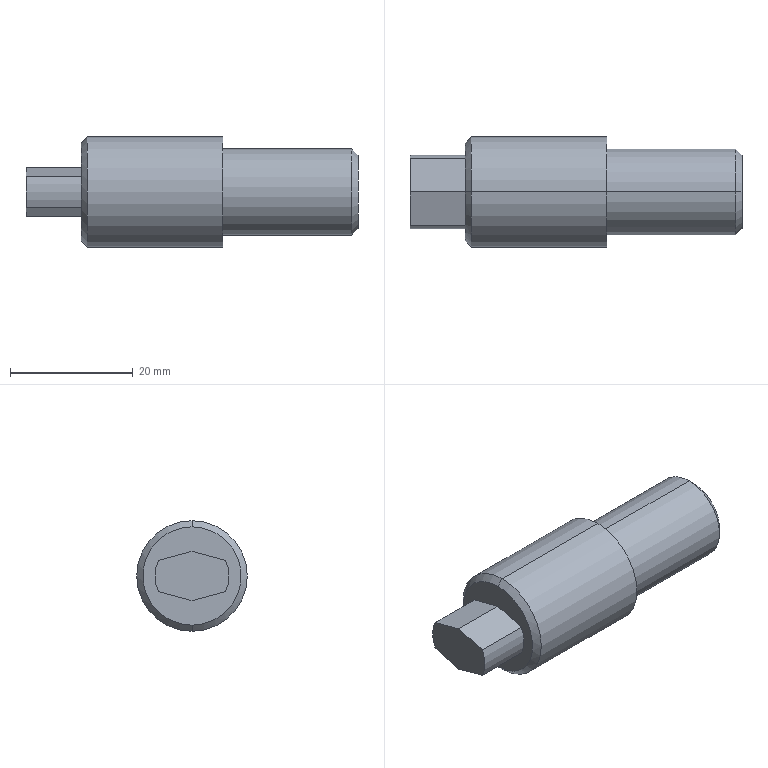Part | SolidWorks | features Chamfer 2, ICE 1, Revolution 1 | 1 solid | 18 faces | box 54 x 18 x 18 mm | volume 9866 mm3 | plane 8 | cylinder 6 | cone 4 | commonest cylinder face diameters 12 x2 14 x2 18 x2
STEP:
#1=CARTESIAN_POINT('',(-21.473,0.,8.));
#2=VERTEX_POINT('',#1);
#3=CARTESIAN_POINT('',(-21.473,0.,-8.));
#4=VERTEX_POINT('',#3);
#5=CARTESIAN_POINT('',(-21.473,0.,0.));
#6=DIRECTION('',(-1.,0.,0.));
#7=DIRECTION('',(0.,0.,-1.));
#8=AXIS2_PLACEMENT_3D('',#5,#6,#7);
#9=CIRCLE('',#8,8.);
#10=EDGE_CURVE('',#2,#4,#9,.T.);
#11=ORIENTED_EDGE('',*,*,#10,.F.);
#12=CARTESIAN_POINT('',(-20.473,0.,9.));
#13=VERTEX_POINT('',#12);
#14=CARTESIAN_POINT('',(-21.473,0.,8.));
#15=DIRECTION('',(0.7071,0.,0.7071));
#16=VECTOR('',#15,1000.);
#17=LINE('',#14,#16);
#18=EDGE_CURVE('',#2,#13,#17,.T.);
#19=ORIENTED_EDGE('',*,*,#18,.T.);
#20=CARTESIAN_POINT('',(-20.473,0.,-9.));
#21=VERTEX_POINT('',#20);
#22=CARTESIAN_POINT('',(-20.473,0.,0.));
#23=DIRECTION('',(1.,0.,0.));
#24=DIRECTION('',(0.,0.,-1.));
#25=AXIS2_PLACEMENT_3D('',#22,#23,#24);
#26=CIRCLE('',#25,9.);
#27=EDGE_CURVE('',#21,#13,#26,.T.);
#28=ORIENTED_EDGE('',*,*,#27,.F.);
#29=CARTESIAN_POINT('',(-21.473,0.,-8.));
#30=DIRECTION('',(0.7071,0.,-0.7071));
#31=VECTOR('',#30,1000.);
#32=LINE('',#29,#31);
#33=EDGE_CURVE('',#4,#21,#32,.T.);
#34=ORIENTED_EDGE('',*,*,#33,.F.);
#35=EDGE_LOOP('',(#11,#19,#28,#34));
#36=FACE_OUTER_BOUND('',#35,.T.);
#37=CARTESIAN_POINT('',(-21.473,0.,0.));
#38=DIRECTION('',(1.,0.,0.));
#39=DIRECTION('',(0.,0.,-1.));
#40=AXIS2_PLACEMENT_3D('',#37,#38,#39);
#41=CONICAL_SURFACE('',#40,8.,0.7854);
#42=ADVANCED_FACE('',(#36),#41,.T.);
#43=CARTESIAN_POINT('',(23.527,0.,-6.));
#44=VERTEX_POINT('',#43);
#45=CARTESIAN_POINT('',(23.527,0.,6.));
#46=VERTEX_POINT('',#45);
#47=CARTESIAN_POINT('',(23.527,0.,0.));
#48=DIRECTION('',(1.,0.,0.));
#49=DIRECTION('',(0.,0.,1.));
#50=AXIS2_PLACEMENT_3D('',#47,#48,#49);
#51=CIRCLE('',#50,6.);
#52=EDGE_CURVE('',#44,#46,#51,.T.);
#53=ORIENTED_EDGE('',*,*,#52,.F.);
#54=CARTESIAN_POINT('',(22.527,0.,-7.));
#55=VERTEX_POINT('',#54);
#56=CARTESIAN_POINT('',(22.527,0.,-7.));
#57=DIRECTION('',(-0.7071,0.,-0.7071));
#58=VECTOR('',#57,1000.);
#59=LINE('',#56,#58);
#60=EDGE_CURVE('',#44,#55,#59,.T.);
#61=ORIENTED_EDGE('',*,*,#60,.T.);
#62=CARTESIAN_POINT('',(22.527,0.,7.));
#63=VERTEX_POINT('',#62);
#64=CARTESIAN_POINT('',(22.527,0.,0.));
#65=DIRECTION('',(-1.,0.,0.));
#66=DIRECTION('',(0.,0.,1.));
#67=AXIS2_PLACEMENT_3D('',#64,#65,#66);
#68=CIRCLE('',#67,7.);
#69=EDGE_CURVE('',#63,#55,#68,.T.);
#70=ORIENTED_EDGE('',*,*,#69,.F.);
#71=CARTESIAN_POINT('',(22.527,0.,7.));
#72=DIRECTION('',(-0.7071,0.,0.7071));
#73=VECTOR('',#72,1000.);
#74=LINE('',#71,#73);
#75=EDGE_CURVE('',#46,#63,#74,.T.);
#76=ORIENTED_EDGE('',*,*,#75,.F.);
#77=EDGE_LOOP('',(#53,#61,#70,#76));
#78=FACE_OUTER_BOUND('',#77,.T.);
#79=CARTESIAN_POINT('',(22.527,0.,0.));
#80=DIRECTION('',(-1.,0.,0.));
#81=DIRECTION('',(0.,0.,1.));
#82=AXIS2_PLACEMENT_3D('',#79,#80,#81);
#83=CONICAL_SURFACE('',#82,7.,0.7854);
#84=ADVANCED_FACE('',(#78),#83,.T.);
#85=ORIENTED_EDGE('',*,*,#69,.T.);
#86=CARTESIAN_POINT('',(1.527,0.,-7.));
#87=VERTEX_POINT('',#86);
#88=CARTESIAN_POINT('',(-65.319,0.,-7.));
#89=DIRECTION('',(-1.,0.,0.));
#90=VECTOR('',#89,1000.);
#91=LINE('',#88,#90);
#92=EDGE_CURVE('',#55,#87,#91,.T.);
#93=ORIENTED_EDGE('',*,*,#92,.T.);
#94=CARTESIAN_POINT('',(1.527,0.,7.));
#95=VERTEX_POINT('',#94);
#96=CARTESIAN_POINT('',(1.527,0.,0.));
#97=DIRECTION('',(-1.,0.,0.));
#98=DIRECTION('',(0.,0.,1.));
#99=AXIS2_PLACEMENT_3D('',#96,#97,#98);
#100=CIRCLE('',#99,7.);
#101=EDGE_CURVE('',#95,#87,#100,.T.);
#102=ORIENTED_EDGE('',*,*,#101,.F.);
#103=CARTESIAN_POINT('',(-65.319,0.,7.));
#104=DIRECTION('',(-1.,0.,0.));
#105=VECTOR('',#104,1000.);
#106=LINE('',#103,#105);
#107=EDGE_CURVE('',#63,#95,#106,.T.);
#108=ORIENTED_EDGE('',*,*,#107,.F.);
#109=EDGE_LOOP('',(#85,#93,#102,#108));
#110=FACE_OUTER_BOUND('',#109,.T.);
#111=CARTESIAN_POINT('',(-65.319,0.,0.));
#112=DIRECTION('',(-1.,0.,0.));
#113=DIRECTION('',(0.,0.,1.));
#114=AXIS2_PLACEMENT_3D('',#111,#112,#113);
#115=CYLINDRICAL_SURFACE('',#114,7.);
#116=ADVANCED_FACE('',(#110),#115,.T.);
#117=CARTESIAN_POINT('',(1.527,0.,9.));
#118=VERTEX_POINT('',#117);
#119=CARTESIAN_POINT('',(1.527,0.,-9.));
#120=VERTEX_POINT('',#119);
#121=CARTESIAN_POINT('',(1.527,0.,0.));
#122=DIRECTION('',(-1.,0.,0.));
#123=DIRECTION('',(0.,0.,1.));
#124=AXIS2_PLACEMENT_3D('',#121,#122,#123);
#125=CIRCLE('',#124,9.);
#126=EDGE_CURVE('',#118,#120,#125,.T.);
#127=ORIENTED_EDGE('',*,*,#126,.T.);
#128=CARTESIAN_POINT('',(-65.319,0.,-9.));
#129=DIRECTION('',(-1.,0.,0.));
#130=VECTOR('',#129,1000.);
#131=LINE('',#128,#130);
#132=EDGE_CURVE('',#120,#21,#131,.T.);
#133=ORIENTED_EDGE('',*,*,#132,.T.);
#134=ORIENTED_EDGE('',*,*,#27,.T.);
#135=CARTESIAN_POINT('',(-65.319,0.,9.));
#136=DIRECTION('',(-1.,0.,0.));
#137=VECTOR('',#136,1000.);
#138=LINE('',#135,#137);
#139=EDGE_CURVE('',#118,#13,#138,.T.);
#140=ORIENTED_EDGE('',*,*,#139,.F.);
#141=EDGE_LOOP('',(#127,#133,#134,#140));
#142=FACE_OUTER_BOUND('',#141,.T.);
#143=CARTESIAN_POINT('',(-65.319,0.,0.));
#144=DIRECTION('',(-1.,0.,0.));
#145=DIRECTION('',(0.,0.,1.));
#146=AXIS2_PLACEMENT_3D('',#143,#144,#145);
#147=CYLINDRICAL_SURFACE('',#146,9.);
#148=ADVANCED_FACE('',(#142),#147,.T.);
#149=CARTESIAN_POINT('',(-21.473,0.,0.));
#150=DIRECTION('',(-1.,0.,0.));
#151=DIRECTION('',(0.,0.,-1.));
#152=AXIS2_PLACEMENT_3D('',#149,#150,#151);
#153=CIRCLE('',#152,8.);
#154=EDGE_CURVE('',#4,#2,#153,.T.);
#155=ORIENTED_EDGE('',*,*,#154,.T.);
#156=ORIENTED_EDGE('',*,*,#10,.T.);
#157=EDGE_LOOP('',(#155,#156));
#158=FACE_OUTER_BOUND('',#157,.T.);
#159=CARTESIAN_POINT('',(-21.473,-5.434,-2.544));
#160=VERTEX_POINT('',#159);
#161=CARTESIAN_POINT('',(-21.473,-5.434,2.544));
#162=VERTEX_POINT('',#161);
#163=CARTESIAN_POINT('',(-21.473,0.,0.));
#164=DIRECTION('',(-1.,0.,0.));
#165=DIRECTION('',(0.,0.,1.));
#166=AXIS2_PLACEMENT_3D('',#163,#164,#165);
#167=CIRCLE('',#166,6.);
#168=EDGE_CURVE('',#160,#162,#167,.T.);
#169=ORIENTED_EDGE('',*,*,#168,.F.);
#170=CARTESIAN_POINT('',(-21.473,0.,-4.));
#171=VERTEX_POINT('',#170);
#172=CARTESIAN_POINT('',(-21.473,0.,-4.));
#173=DIRECTION('',(0.,-0.9659,0.2588));
#174=VECTOR('',#173,1000.);
#175=LINE('',#172,#174);
#176=EDGE_CURVE('',#171,#160,#175,.T.);
#177=ORIENTED_EDGE('',*,*,#176,.F.);
#178=CARTESIAN_POINT('',(-21.473,5.434,-2.544));
#179=VERTEX_POINT('',#178);
#180=CARTESIAN_POINT('',(-21.473,0.,-4.));
#181=DIRECTION('',(0.,-0.9659,-0.2588));
#182=VECTOR('',#181,1000.);
#183=LINE('',#180,#182);
#184=EDGE_CURVE('',#179,#171,#183,.T.);
#185=ORIENTED_EDGE('',*,*,#184,.F.);
#186=CARTESIAN_POINT('',(-21.473,5.434,2.544));
#187=VERTEX_POINT('',#186);
#188=CARTESIAN_POINT('',(-21.473,0.,0.));
#189=DIRECTION('',(-1.,0.,0.));
#190=DIRECTION('',(0.,0.,1.));
#191=AXIS2_PLACEMENT_3D('',#188,#189,#190);
#192=CIRCLE('',#191,6.);
#193=EDGE_CURVE('',#187,#179,#192,.T.);
#194=ORIENTED_EDGE('',*,*,#193,.F.);
#195=CARTESIAN_POINT('',(-21.473,0.,4.));
#196=VERTEX_POINT('',#195);
#197=CARTESIAN_POINT('',(-21.473,0.,4.));
#198=DIRECTION('',(0.,0.9659,-0.2588));
#199=VECTOR('',#198,1000.);
#200=LINE('',#197,#199);
#201=EDGE_CURVE('',#196,#187,#200,.T.);
#202=ORIENTED_EDGE('',*,*,#201,.F.);
#203=CARTESIAN_POINT('',(-21.473,0.,4.));
#204=DIRECTION('',(0.,0.9659,0.2588));
#205=VECTOR('',#204,1000.);
#206=LINE('',#203,#205);
#207=EDGE_CURVE('',#162,#196,#206,.T.);
#208=ORIENTED_EDGE('',*,*,#207,.F.);
#209=EDGE_LOOP('',(#169,#177,#185,#194,#202,#208));
#210=FACE_BOUND('',#209,.T.);
#211=CARTESIAN_POINT('',(-21.473,0.,0.));
#212=DIRECTION('',(1.,0.,0.));
#213=DIRECTION('',(0.,0.,-1.));
#214=AXIS2_PLACEMENT_3D('',#211,#212,#213);
#215=PLANE('',#214);
#216=ADVANCED_FACE('',(#158,#210),#215,.F.);
#217=ORIENTED_EDGE('',*,*,#132,.F.);
#218=CARTESIAN_POINT('',(1.527,0.,0.));
#219=DIRECTION('',(-1.,0.,0.));
#220=DIRECTION('',(0.,0.,1.));
#221=AXIS2_PLACEMENT_3D('',#218,#219,#220);
#222=CIRCLE('',#221,9.);
#223=EDGE_CURVE('',#120,#118,#222,.T.);
#224=ORIENTED_EDGE('',*,*,#223,.T.);
#225=ORIENTED_EDGE('',*,*,#139,.T.);
#226=CARTESIAN_POINT('',(-20.473,0.,0.));
#227=DIRECTION('',(1.,0.,0.));
#228=DIRECTION('',(0.,0.,-1.));
#229=AXIS2_PLACEMENT_3D('',#226,#227,#228);
#230=CIRCLE('',#229,9.);
#231=EDGE_CURVE('',#13,#21,#230,.T.);
#232=ORIENTED_EDGE('',*,*,#231,.T.);
#233=EDGE_LOOP('',(#217,#224,#225,#232));
#234=FACE_OUTER_BOUND('',#233,.T.);
#235=CARTESIAN_POINT('',(-65.319,0.,0.));
#236=DIRECTION('',(-1.,0.,0.));
#237=DIRECTION('',(0.,0.,1.));
#238=AXIS2_PLACEMENT_3D('',#235,#236,#237);
#239=CYLINDRICAL_SURFACE('',#238,9.);
#240=ADVANCED_FACE('',(#234),#239,.T.);
#241=ORIENTED_EDGE('',*,*,#126,.F.);
#242=ORIENTED_EDGE('',*,*,#223,.F.);
#243=EDGE_LOOP('',(#241,#242));
#244=FACE_OUTER_BOUND('',#243,.T.);
#245=ORIENTED_EDGE('',*,*,#101,.T.);
#246=CARTESIAN_POINT('',(1.527,0.,0.));
#247=DIRECTION('',(-1.,0.,0.));
#248=DIRECTION('',(0.,0.,1.));
#249=AXIS2_PLACEMENT_3D('',#246,#247,#248);
#250=CIRCLE('',#249,7.);
#251=EDGE_CURVE('',#87,#95,#250,.T.);
#252=ORIENTED_EDGE('',*,*,#251,.T.);
#253=EDGE_LOOP('',(#245,#252));
#254=FACE_BOUND('',#253,.T.);
#255=CARTESIAN_POINT('',(1.527,9.,0.));
#256=DIRECTION('',(-1.,0.,0.));
#257=DIRECTION('',(0.,0.,1.));
#258=AXIS2_PLACEMENT_3D('',#255,#256,#257);
#259=PLANE('',#258);
#260=ADVANCED_FACE('',(#244,#254),#259,.F.);
#261=ORIENTED_EDGE('',*,*,#92,.F.);
#262=CARTESIAN_POINT('',(22.527,0.,0.));
#263=DIRECTION('',(-1.,0.,0.));
#264=DIRECTION('',(0.,0.,1.));
#265=AXIS2_PLACEMENT_3D('',#262,#263,#264);
#266=CIRCLE('',#265,7.);
#267=EDGE_CURVE('',#55,#63,#266,.T.);
#268=ORIENTED_EDGE('',*,*,#267,.T.);
#269=ORIENTED_EDGE('',*,*,#107,.T.);
#270=ORIENTED_EDGE('',*,*,#251,.F.);
#271=EDGE_LOOP('',(#261,#268,#269,#270));
#272=FACE_OUTER_BOUND('',#271,.T.);
#273=CARTESIAN_POINT('',(-65.319,0.,0.));
#274=DIRECTION('',(-1.,0.,0.));
#275=DIRECTION('',(0.,0.,1.));
#276=AXIS2_PLACEMENT_3D('',#273,#274,#275);
#277=CYLINDRICAL_SURFACE('',#276,7.);
#278=ADVANCED_FACE('',(#272),#277,.T.);
#279=CARTESIAN_POINT('',(23.527,0.,0.));
#280=DIRECTION('',(1.,0.,0.));
#281=DIRECTION('',(0.,0.,1.));
#282=AXIS2_PLACEMENT_3D('',#279,#280,#281);
#283=CIRCLE('',#282,6.);
#284=EDGE_CURVE('',#46,#44,#283,.T.);
#285=ORIENTED_EDGE('',*,*,#284,.T.);
#286=ORIENTED_EDGE('',*,*,#52,.T.);
#287=EDGE_LOOP('',(#285,#286));
#288=FACE_OUTER_BOUND('',#287,.T.);
#289=CARTESIAN_POINT('',(23.527,7.,0.));
#290=DIRECTION('',(-1.,0.,0.));
#291=DIRECTION('',(0.,0.,1.));
#292=AXIS2_PLACEMENT_3D('',#289,#290,#291);
#293=PLANE('',#292);
#294=ADVANCED_FACE('',(#288),#293,.F.);
#295=ORIENTED_EDGE('',*,*,#60,.F.);
#296=ORIENTED_EDGE('',*,*,#284,.F.);
#297=ORIENTED_EDGE('',*,*,#75,.T.);
#298=ORIENTED_EDGE('',*,*,#267,.F.);
#299=EDGE_LOOP('',(#295,#296,#297,#298));
#300=FACE_OUTER_BOUND('',#299,.T.);
#301=CARTESIAN_POINT('',(22.527,0.,0.));
#302=DIRECTION('',(-1.,0.,0.));
#303=DIRECTION('',(0.,0.,1.));
#304=AXIS2_PLACEMENT_3D('',#301,#302,#303);
#305=CONICAL_SURFACE('',#304,7.,0.7854);
#306=ADVANCED_FACE('',(#300),#305,.T.);
#307=ORIENTED_EDGE('',*,*,#18,.F.);
#308=ORIENTED_EDGE('',*,*,#154,.F.);
#309=ORIENTED_EDGE('',*,*,#33,.T.);
#310=ORIENTED_EDGE('',*,*,#231,.F.);
#311=EDGE_LOOP('',(#307,#308,#309,#310));
#312=FACE_OUTER_BOUND('',#311,.T.);
#313=CARTESIAN_POINT('',(-21.473,0.,0.));
#314=DIRECTION('',(1.,0.,0.));
#315=DIRECTION('',(0.,0.,-1.));
#316=AXIS2_PLACEMENT_3D('',#313,#314,#315);
#317=CONICAL_SURFACE('',#316,8.,0.7854);
#318=ADVANCED_FACE('',(#312),#317,.T.);
#319=ORIENTED_EDGE('',*,*,#168,.T.);
#320=CARTESIAN_POINT('',(-30.473,-5.434,2.544));
#321=VERTEX_POINT('',#320);
#322=CARTESIAN_POINT('',(-30.473,-5.434,2.544));
#323=DIRECTION('',(1.,0.,0.));
#324=VECTOR('',#323,1000.);
#325=LINE('',#322,#324);
#326=EDGE_CURVE('',#321,#162,#325,.T.);
#327=ORIENTED_EDGE('',*,*,#326,.F.);
#328=CARTESIAN_POINT('',(-30.473,-5.434,-2.544));
#329=VERTEX_POINT('',#328);
#330=CARTESIAN_POINT('',(-30.473,0.,0.));
#331=DIRECTION('',(-1.,0.,0.));
#332=DIRECTION('',(0.,0.,1.));
#333=AXIS2_PLACEMENT_3D('',#330,#331,#332);
#334=CIRCLE('',#333,6.);
#335=EDGE_CURVE('',#329,#321,#334,.T.);
#336=ORIENTED_EDGE('',*,*,#335,.F.);
#337=CARTESIAN_POINT('',(-30.473,-5.434,-2.544));
#338=DIRECTION('',(1.,0.,0.));
#339=VECTOR('',#338,1000.);
#340=LINE('',#337,#339);
#341=EDGE_CURVE('',#329,#160,#340,.T.);
#342=ORIENTED_EDGE('',*,*,#341,.T.);
#343=EDGE_LOOP('',(#319,#327,#336,#342));
#344=FACE_OUTER_BOUND('',#343,.T.);
#345=CARTESIAN_POINT('',(-30.473,0.,0.));
#346=DIRECTION('',(1.,0.,0.));
#347=DIRECTION('',(0.,0.,-1.));
#348=AXIS2_PLACEMENT_3D('',#345,#346,#347);
#349=CYLINDRICAL_SURFACE('',#348,6.);
#350=ADVANCED_FACE('',(#344),#349,.T.);
#351=ORIENTED_EDGE('',*,*,#207,.T.);
#352=CARTESIAN_POINT('',(-30.473,0.,4.));
#353=VERTEX_POINT('',#352);
#354=CARTESIAN_POINT('',(-30.473,0.,4.));
#355=DIRECTION('',(1.,0.,0.));
#356=VECTOR('',#355,1000.);
#357=LINE('',#354,#356);
#358=EDGE_CURVE('',#353,#196,#357,.T.);
#359=ORIENTED_EDGE('',*,*,#358,.F.);
#360=CARTESIAN_POINT('',(-30.473,0.,4.));
#361=DIRECTION('',(0.,0.9659,0.2588));
#362=VECTOR('',#361,1000.);
#363=LINE('',#360,#362);
#364=EDGE_CURVE('',#321,#353,#363,.T.);
#365=ORIENTED_EDGE('',*,*,#364,.F.);
#366=ORIENTED_EDGE('',*,*,#326,.T.);
#367=EDGE_LOOP('',(#351,#359,#365,#366));
#368=FACE_OUTER_BOUND('',#367,.T.);
#369=CARTESIAN_POINT('',(-30.473,0.,4.));
#370=DIRECTION('',(0.,0.2588,-0.9659));
#371=DIRECTION('',(0.,0.9659,0.2588));
#372=AXIS2_PLACEMENT_3D('',#369,#370,#371);
#373=PLANE('',#372);
#374=ADVANCED_FACE('',(#368),#373,.F.);
#375=ORIENTED_EDGE('',*,*,#201,.T.);
#376=CARTESIAN_POINT('',(-30.473,5.434,2.544));
#377=VERTEX_POINT('',#376);
#378=CARTESIAN_POINT('',(-30.473,5.434,2.544));
#379=DIRECTION('',(1.,0.,0.));
#380=VECTOR('',#379,1000.);
#381=LINE('',#378,#380);
#382=EDGE_CURVE('',#377,#187,#381,.T.);
#383=ORIENTED_EDGE('',*,*,#382,.F.);
#384=CARTESIAN_POINT('',(-30.473,0.,4.));
#385=DIRECTION('',(0.,0.9659,-0.2588));
#386=VECTOR('',#385,1000.);
#387=LINE('',#384,#386);
#388=EDGE_CURVE('',#353,#377,#387,.T.);
#389=ORIENTED_EDGE('',*,*,#388,.F.);
#390=ORIENTED_EDGE('',*,*,#358,.T.);
#391=EDGE_LOOP('',(#375,#383,#389,#390));
#392=FACE_OUTER_BOUND('',#391,.T.);
#393=CARTESIAN_POINT('',(-30.473,0.,4.));
#394=DIRECTION('',(0.,-0.2588,-0.9659));
#395=DIRECTION('',(0.,0.9659,-0.2588));
#396=AXIS2_PLACEMENT_3D('',#393,#394,#395);
#397=PLANE('',#396);
#398=ADVANCED_FACE('',(#392),#397,.F.);
#399=ORIENTED_EDGE('',*,*,#193,.T.);
#400=CARTESIAN_POINT('',(-30.473,5.434,-2.544));
#401=VERTEX_POINT('',#400);
#402=CARTESIAN_POINT('',(-30.473,5.434,-2.544));
#403=DIRECTION('',(1.,0.,0.));
#404=VECTOR('',#403,1000.);
#405=LINE('',#402,#404);
#406=EDGE_CURVE('',#401,#179,#405,.T.);
#407=ORIENTED_EDGE('',*,*,#406,.F.);
#408=CARTESIAN_POINT('',(-30.473,0.,0.));
#409=DIRECTION('',(-1.,0.,0.));
#410=DIRECTION('',(0.,0.,1.));
#411=AXIS2_PLACEMENT_3D('',#408,#409,#410);
#412=CIRCLE('',#411,6.);
#413=EDGE_CURVE('',#377,#401,#412,.T.);
#414=ORIENTED_EDGE('',*,*,#413,.F.);
#415=ORIENTED_EDGE('',*,*,#382,.T.);
#416=EDGE_LOOP('',(#399,#407,#414,#415));
#417=FACE_OUTER_BOUND('',#416,.T.);
#418=CARTESIAN_POINT('',(-30.473,0.,0.));
#419=DIRECTION('',(1.,0.,0.));
#420=DIRECTION('',(0.,0.,-1.));
#421=AXIS2_PLACEMENT_3D('',#418,#419,#420);
#422=CYLINDRICAL_SURFACE('',#421,6.);
#423=ADVANCED_FACE('',(#417),#422,.T.);
#424=ORIENTED_EDGE('',*,*,#184,.T.);
#425=CARTESIAN_POINT('',(-30.473,0.,-4.));
#426=VERTEX_POINT('',#425);
#427=CARTESIAN_POINT('',(-30.473,0.,-4.));
#428=DIRECTION('',(1.,0.,0.));
#429=VECTOR('',#428,1000.);
#430=LINE('',#427,#429);
#431=EDGE_CURVE('',#426,#171,#430,.T.);
#432=ORIENTED_EDGE('',*,*,#431,.F.);
#433=CARTESIAN_POINT('',(-30.473,0.,-4.));
#434=DIRECTION('',(0.,-0.9659,-0.2588));
#435=VECTOR('',#434,1000.);
#436=LINE('',#433,#435);
#437=EDGE_CURVE('',#401,#426,#436,.T.);
#438=ORIENTED_EDGE('',*,*,#437,.F.);
#439=ORIENTED_EDGE('',*,*,#406,.T.);
#440=EDGE_LOOP('',(#424,#432,#438,#439));
#441=FACE_OUTER_BOUND('',#440,.T.);
#442=CARTESIAN_POINT('',(-30.473,0.,-4.));
#443=DIRECTION('',(0.,-0.2588,0.9659));
#444=DIRECTION('',(0.,-0.9659,-0.2588));
#445=AXIS2_PLACEMENT_3D('',#442,#443,#444);
#446=PLANE('',#445);
#447=ADVANCED_FACE('',(#441),#446,.F.);
#448=ORIENTED_EDGE('',*,*,#176,.T.);
#449=ORIENTED_EDGE('',*,*,#341,.F.);
#450=CARTESIAN_POINT('',(-30.473,0.,-4.));
#451=DIRECTION('',(0.,-0.9659,0.2588));
#452=VECTOR('',#451,1000.);
#453=LINE('',#450,#452);
#454=EDGE_CURVE('',#426,#329,#453,.T.);
#455=ORIENTED_EDGE('',*,*,#454,.F.);
#456=ORIENTED_EDGE('',*,*,#431,.T.);
#457=EDGE_LOOP('',(#448,#449,#455,#456));
#458=FACE_OUTER_BOUND('',#457,.T.);
#459=CARTESIAN_POINT('',(-30.473,0.,-4.));
#460=DIRECTION('',(0.,0.2588,0.9659));
#461=DIRECTION('',(0.,-0.9659,0.2588));
#462=AXIS2_PLACEMENT_3D('',#459,#460,#461);
#463=PLANE('',#462);
#464=ADVANCED_FACE('',(#458),#463,.F.);
#465=ORIENTED_EDGE('',*,*,#335,.T.);
#466=ORIENTED_EDGE('',*,*,#364,.T.);
#467=ORIENTED_EDGE('',*,*,#388,.T.);
#468=ORIENTED_EDGE('',*,*,#413,.T.);
#469=ORIENTED_EDGE('',*,*,#437,.T.);
#470=ORIENTED_EDGE('',*,*,#454,.T.);
#471=EDGE_LOOP('',(#465,#466,#467,#468,#469,#470));
#472=FACE_OUTER_BOUND('',#471,.T.);
#473=CARTESIAN_POINT('',(-30.473,0.,0.));
#474=DIRECTION('',(-1.,0.,0.));
#475=DIRECTION('',(0.,0.,1.));
#476=AXIS2_PLACEMENT_3D('',#473,#474,#475);
#477=PLANE('',#476);
#478=ADVANCED_FACE('',(#472),#477,.T.);
#479=CLOSED_SHELL('',(#42,#84,#116,#148,#216,#240,#260,#278,#294,#306,#318,#350,#374,#398,#423,#447,#464,#478));
#480=MANIFOLD_SOLID_BREP('',#479);
#481=CARTESIAN_POINT('',(0.,0.,0.));
#482=DIRECTION('',(0.,0.,1.));
#483=DIRECTION('',(1.,0.,0.));
#484=AXIS2_PLACEMENT_3D('',#481,#482,#483);
#485=(LENGTH_UNIT()NAMED_UNIT(*)SI_UNIT(.MILLI.,.METRE.));
#486=UNCERTAINTY_MEASURE_WITH_UNIT(LENGTH_MEASURE(0.00001),#485,'','');
#487=(NAMED_UNIT(*)PLANE_ANGLE_UNIT()SI_UNIT($,.RADIAN.));
#488=(NAMED_UNIT(*)SI_UNIT($,.STERADIAN.)SOLID_ANGLE_UNIT());
#489=(GEOMETRIC_REPRESENTATION_CONTEXT(3)GLOBAL_UNCERTAINTY_ASSIGNED_CONTEXT((#486))GLOBAL_UNIT_ASSIGNED_CONTEXT((#485,#487,#488))REPRESENTATION_CONTEXT('',''));
#490=ADVANCED_BREP_SHAPE_REPRESENTATION('',(#480,#484),#489);